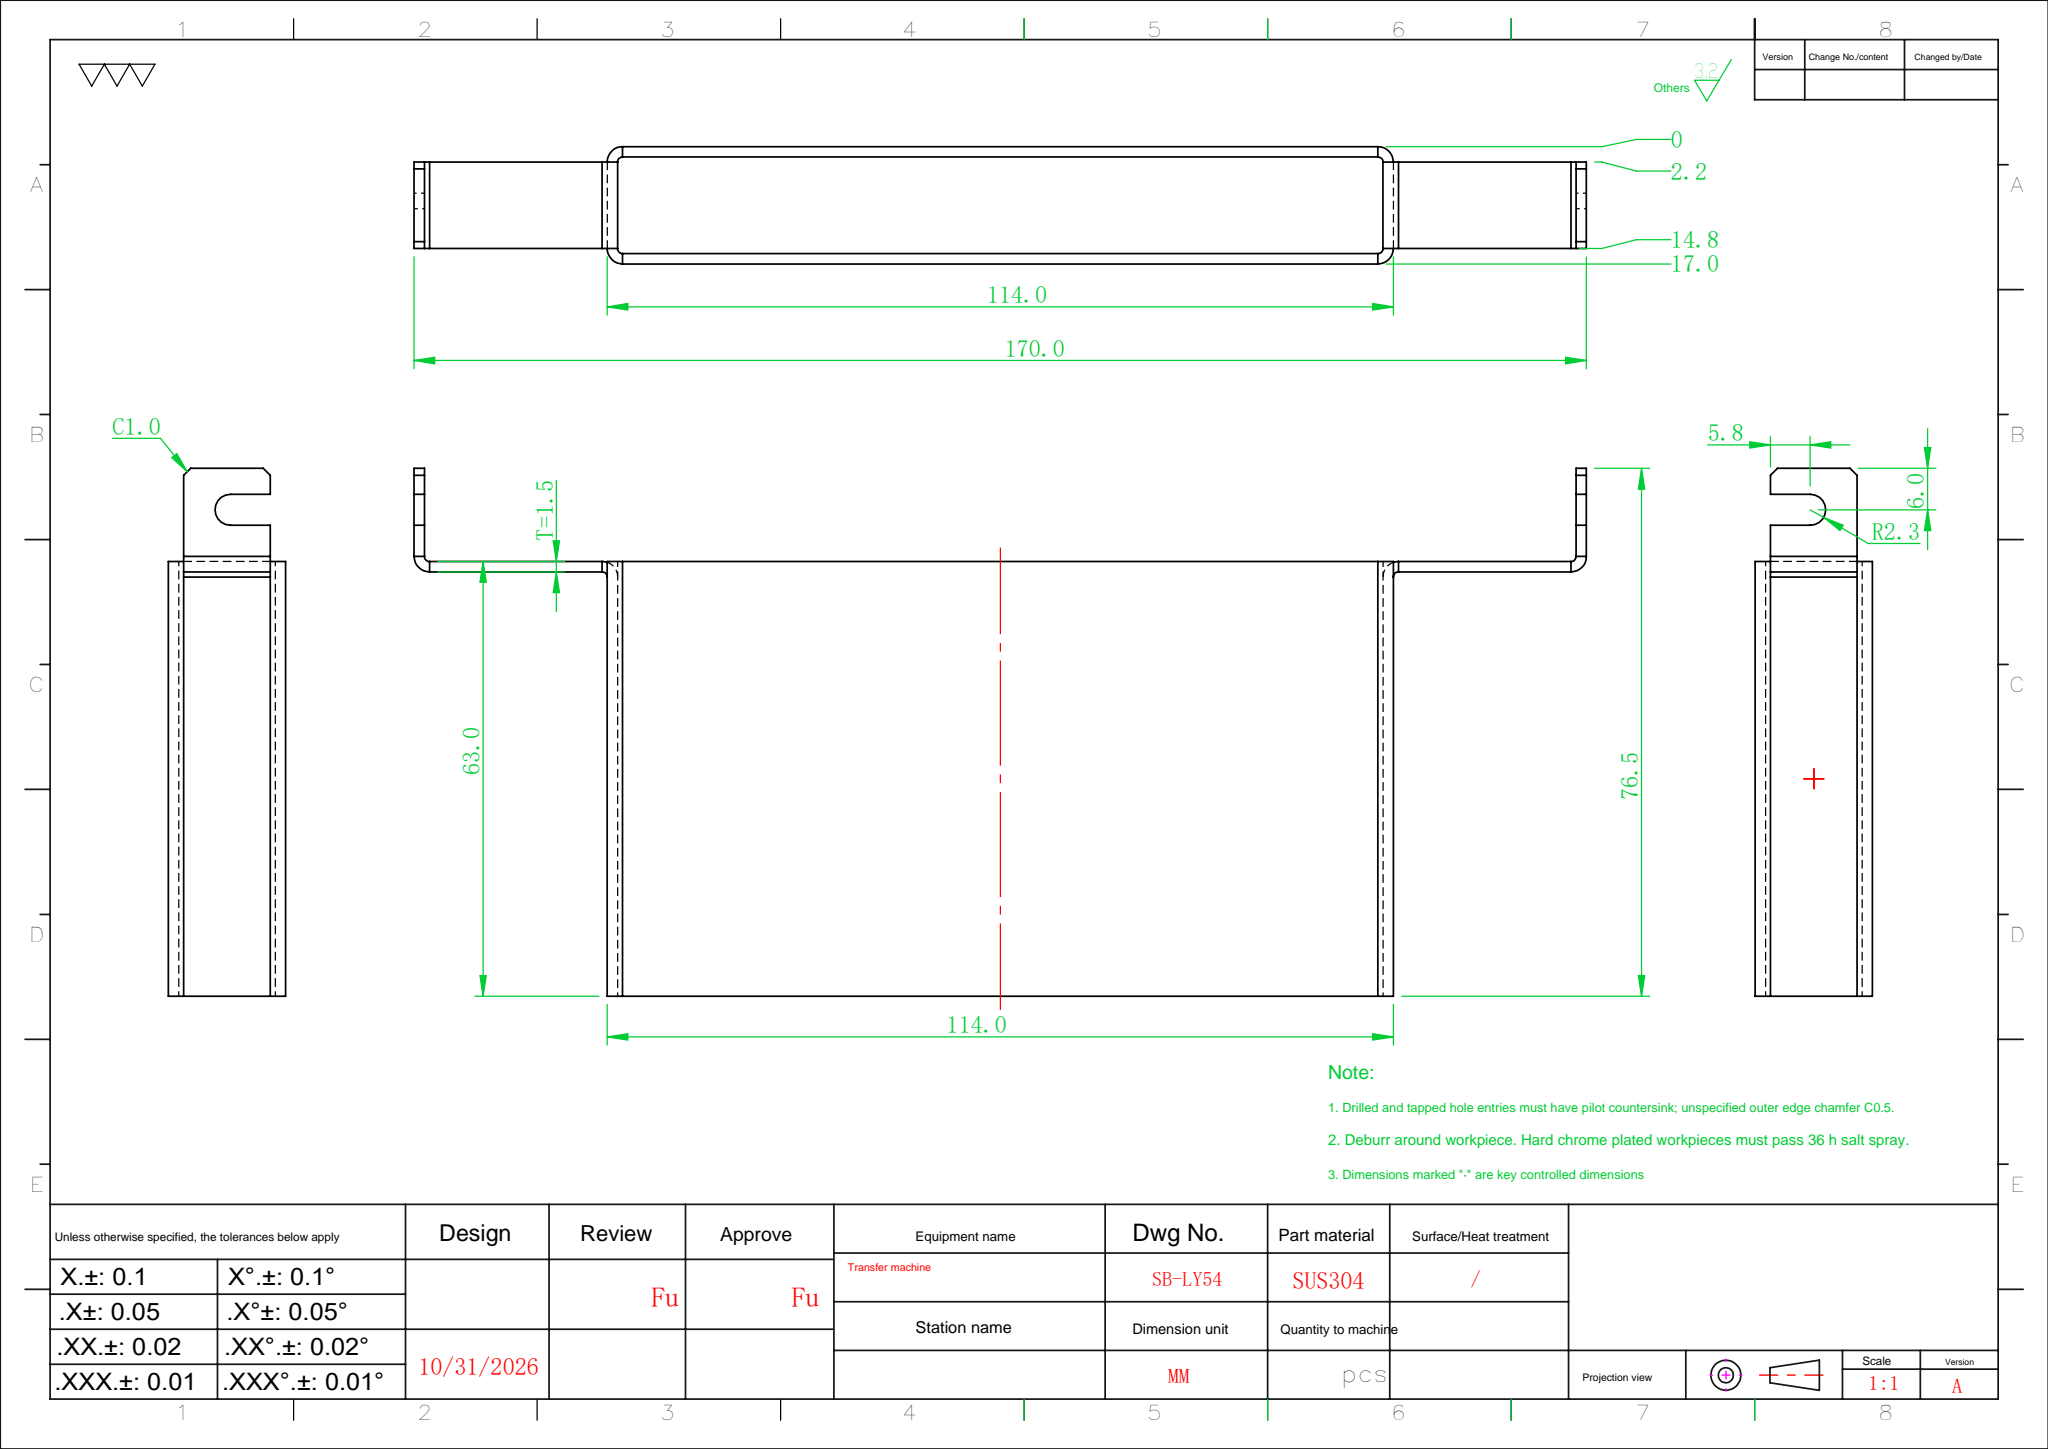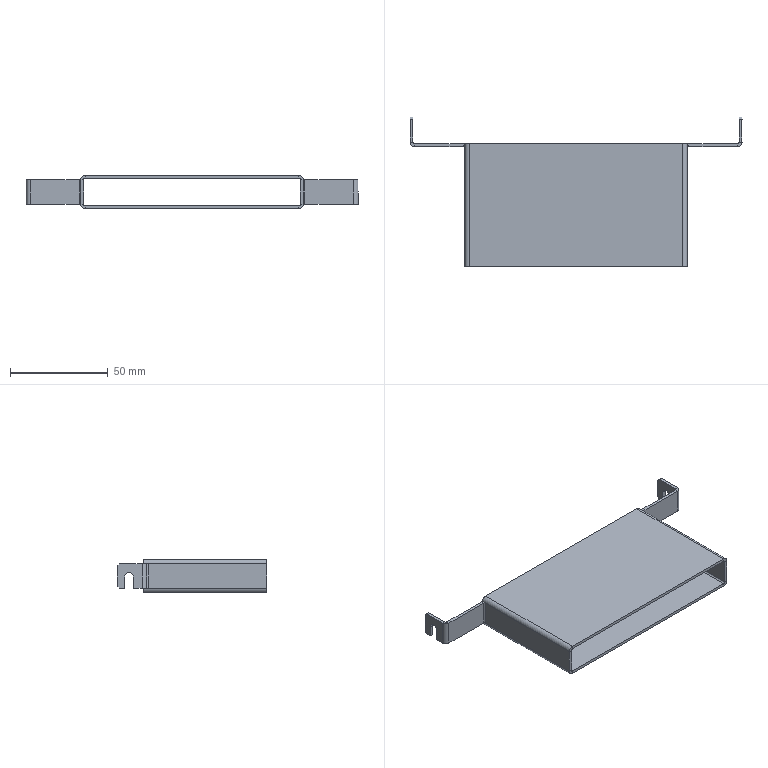Part | SolidWorks | features EdgeFlange 4, SMBaseFlange 2, Chamfer 1, FlatPattern 1, HoleWzd 1, SheetMetal 1 | 1 solid | 80 faces | box 170.003 x 76.5 x 17.003 mm | volume 25360 mm3 | plane 62 | cylinder 18 | commonest cylinder face diameters 1.473 x8 4.473 x8 4.5 x2